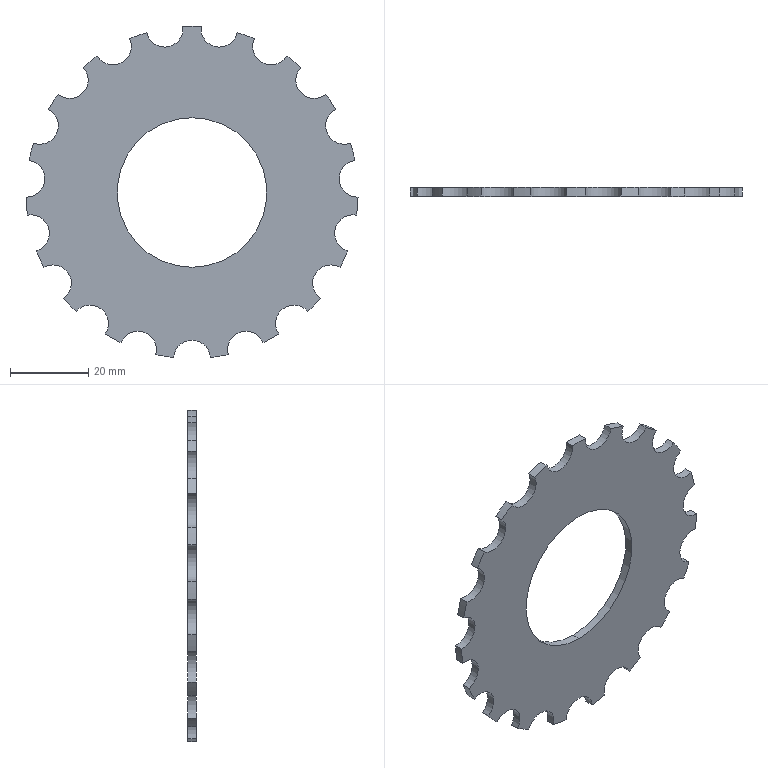Part | STEP file | Gear 3 | 1 solid | 51 faces | box 84.766 x 2.2 x 84.54 mm | volume 8488 mm3 | cylinder 49 | plane 2 | commonest cylinder face diameters 9.4 x28 84.8 x19 38.2 x2